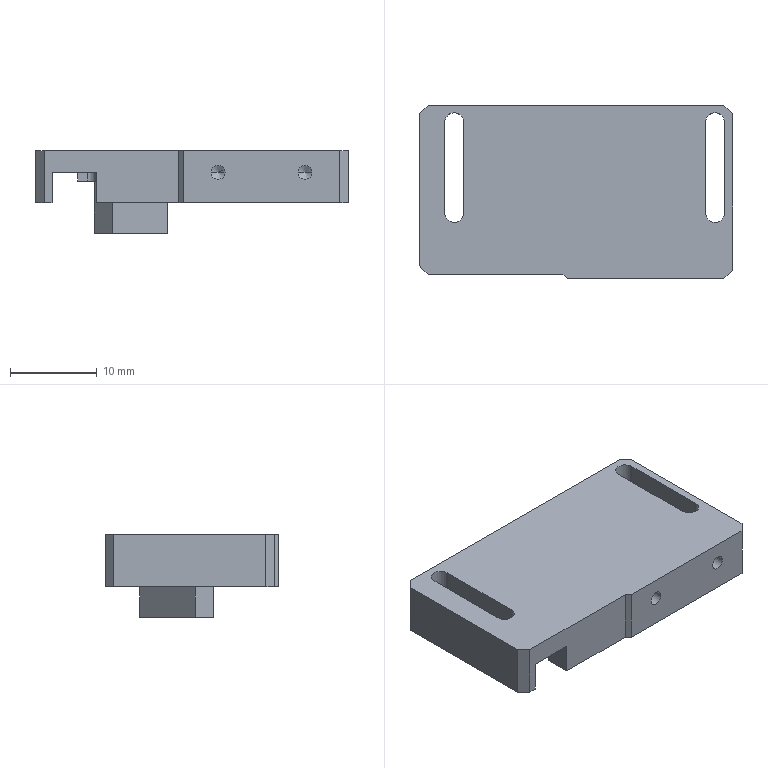NC program | NX | posted with a generic post | part box 36 x 20 x 9.5 mm
Lines 1630 to 2686 of 4561:
(CAVITY_MILL_COPY_COPY , TOOL : D2)
N3240 T02 M6
N3242 G54
N3244 G17 G0 G90 X9.747 Y2.177 S9974 M3
N3246 G43 Z30. H2
N3248 Z-2.092
N3250 G94 G1 Z-3.592 F1000.
N3252 X10.383 Y3.006
N3254 G3 X10.514 Y3.997 R1.
N3256 G1 X11.345 Y4.341
N3258 X11.406 Y4.178
N3260 X11.728 Y4.5
N3262 X11.273
N3264 X11.345 Y4.341
N3266 X10.514 Y3.997
N3268 G2 X10.408 Y2.593 R1.56
N3270 G3 X10.482 Y1.981 R0.5
N3272 G1 X13.122 Y4.621
N3274 G2 X14.745 Y4.548 R1.1
N3276 X15. Y3.828 R1.1
N3278 G1 Y3.39
N3280 G3 X15.485 Y3.771 R0.5
N3282 G2 X16.626 Y4.915 R1.56
N3284 G3 X17.006 Y5.4 R0.5
N3286 G1 X9.066
N3288 G3 X9.446 Y4.915 R0.5
N3290 G2 X10.514 Y3.997 R1.56
N3292 X10.383 Y3.006 R1.
N3294 G1 X9.747 Y2.177
N3296 Z-2.092
N3298 G0 Z-2.285
N3300 G1 Z-3.785
N3302 X10.383 Y3.006
N3304 G3 X10.514 Y3.997 R1.
N3306 G1 X11.345 Y4.341
N3308 X11.406 Y4.178
N3310 X11.728 Y4.5
N3312 X11.273
N3314 X11.345 Y4.341
N3316 X10.514 Y3.997
N3318 G2 X10.408 Y2.593 R1.56
N3320 G3 X10.482 Y1.981 R0.5
N3322 G1 X13.122 Y4.621
N3324 G2 X14.745 Y4.548 R1.1
N3326 X15. Y3.828 R1.1
N3328 G1 Y3.39
N3330 G3 X15.485 Y3.771 R0.5
N3332 G2 X16.626 Y4.915 R1.56
N3334 G3 X17.006 Y5.4 R0.5
N3336 G1 X9.066
N3338 G3 X9.446 Y4.915 R0.5
N3340 G2 X10.514 Y3.997 R1.56
N3342 X10.383 Y3.006 R1.
N3344 G1 X9.747 Y2.177
N3346 Z-2.285
N3348 G0 Z-2.477
N3350 G1 Z-3.977
N3352 X10.383 Y3.006
N3354 G3 X10.514 Y3.997 R1.
N3356 G1 X11.345 Y4.341
N3358 X11.406 Y4.178
N3360 X11.728 Y4.5
N3362 X11.273
N3364 X11.345 Y4.341
N3366 X10.514 Y3.997
N3368 G2 X10.408 Y2.593 R1.56
N3370 G3 X10.482 Y1.981 R0.5
N3372 G1 X13.122 Y4.621
N3374 G2 X14.745 Y4.548 R1.1
N3376 X15. Y3.828 R1.1
N3378 G1 Y3.39
N3380 G3 X15.485 Y3.771 R0.5
N3382 G2 X16.626 Y4.915 R1.56
N3384 G3 X17.006 Y5.4 R0.5
N3386 G1 X9.066
N3388 G3 X9.446 Y4.915 R0.5
N3390 G2 X10.514 Y3.997 R1.56
N3392 X10.383 Y3.006 R1.
N3394 G1 X9.747 Y2.177
N3396 Z-2.477
N3398 G0 Z-2.669
N3400 G1 Z-4.169
N3402 X10.383 Y3.006
N3404 G3 X10.514 Y3.997 R1.
N3406 G1 X11.345 Y4.341
N3408 X11.406 Y4.178
N3410 X11.728 Y4.5
N3412 X11.273
N3414 X11.345 Y4.341
N3416 X10.514 Y3.997
N3418 G2 X10.408 Y2.593 R1.56
N3420 G3 X10.482 Y1.981 R0.5
N3422 G1 X13.122 Y4.621
N3424 G2 X14.745 Y4.548 R1.1
N3426 X15. Y3.828 R1.1
N3428 G1 Y3.39
N3430 G3 X15.485 Y3.771 R0.5
N3432 G2 X16.626 Y4.915 R1.56
N3434 G3 X17.006 Y5.4 R0.5
N3436 G1 X9.066
N3438 G3 X9.446 Y4.915 R0.5
N3440 G2 X10.514 Y3.997 R1.56
N3442 X10.383 Y3.006 R1.
N3444 G1 X9.747 Y2.177
N3446 Z-2.669
N3448 G0 Z-2.862
N3450 G1 Z-4.362
N3452 X10.383 Y3.006
N3454 G3 X10.514 Y3.997 R1.
N3456 G1 X11.345 Y4.341
N3458 X11.406 Y4.178
N3460 X11.728 Y4.5
N3462 X11.273
N3464 X11.345 Y4.341
N3466 X10.514 Y3.997
N3468 G2 X10.408 Y2.593 R1.56
N3470 G3 X10.482 Y1.981 R0.5
N3472 G1 X13.122 Y4.621
N3474 G2 X14.745 Y4.548 R1.1
N3476 X15. Y3.828 R1.1
N3478 G1 Y3.39
N3480 G3 X15.485 Y3.771 R0.5
N3482 G2 X16.626 Y4.915 R1.56
N3484 G3 X17.006 Y5.4 R0.5
N3486 G1 X9.066
N3488 G3 X9.446 Y4.915 R0.5
N3490 G2 X10.514 Y3.997 R1.56
N3492 X10.383 Y3.006 R1.
N3494 G1 X9.747 Y2.177
N3496 Z-2.862
N3498 G0 Z-3.054
N3500 G1 Z-4.554
N3502 X10.383 Y3.006
N3504 G3 X10.514 Y3.997 R1.
N3506 G1 X11.345 Y4.341
N3508 X11.406 Y4.178
N3510 X11.728 Y4.5
N3512 X11.273
N3514 X11.345 Y4.341
N3516 X10.514 Y3.997
N3518 G2 X10.408 Y2.593 R1.56
N3520 G3 X10.482 Y1.981 R0.5
N3522 G1 X13.122 Y4.621
N3524 G2 X14.745 Y4.548 R1.1
N3526 X15. Y3.828 R1.1
N3528 G1 Y3.39
N3530 G3 X15.485 Y3.771 R0.5
N3532 G2 X16.626 Y4.915 R1.56
N3534 G3 X17.006 Y5.4 R0.5
N3536 G1 X9.066
N3538 G3 X9.446 Y4.915 R0.5
N3540 G2 X10.514 Y3.997 R1.56
N3542 X10.383 Y3.006 R1.
N3544 G1 X9.747 Y2.177
N3546 Z-3.054
N3548 G0 Z-3.246
N3550 G1 Z-4.746
N3552 X10.383 Y3.006
N3554 G3 X10.514 Y3.997 R1.
N3556 G1 X11.345 Y4.341
N3558 X11.406 Y4.178
N3560 X11.728 Y4.5
N3562 X11.273
N3564 X11.345 Y4.341
N3566 X10.514 Y3.997
N3568 G2 X10.408 Y2.593 R1.56
N3570 G3 X10.482 Y1.981 R0.5
N3572 G1 X13.122 Y4.621
N3574 G2 X14.745 Y4.548 R1.1
N3576 X15. Y3.828 R1.1
N3578 G1 Y3.39
N3580 G3 X15.485 Y3.771 R0.5
N3582 G2 X16.626 Y4.915 R1.56
N3584 G3 X17.006 Y5.4 R0.5
N3586 G1 X9.066
N3588 G3 X9.446 Y4.915 R0.5
N3590 G2 X10.514 Y3.997 R1.56
N3592 X10.383 Y3.006 R1.
N3594 G1 X9.747 Y2.177
N3596 Z-3.246
N3598 G0 Z-3.438
N3600 G1 Z-4.938
N3602 X10.383 Y3.006
N3604 G3 X10.514 Y3.997 R1.
N3606 G1 X11.345 Y4.341
N3608 X11.406 Y4.178
N3610 X11.728 Y4.5
N3612 X11.273
N3614 X11.345 Y4.341
N3616 X10.514 Y3.997
N3618 G2 X10.408 Y2.593 R1.56
N3620 G3 X10.482 Y1.981 R0.5
N3622 G1 X13.122 Y4.621
N3624 G2 X14.745 Y4.548 R1.1
N3626 X15. Y3.828 R1.1
N3628 G1 Y3.39
N3630 G3 X15.485 Y3.771 R0.5
N3632 G2 X16.626 Y4.915 R1.56
N3634 G3 X17.006 Y5.4 R0.5
N3636 G1 X9.066
N3638 G3 X9.446 Y4.915 R0.5
N3640 G2 X10.514 Y3.997 R1.56
N3642 X10.383 Y3.006 R1.
N3644 G1 X9.747 Y2.177
N3646 Z-3.438
N3648 G0 Z-3.631
N3650 G1 Z-5.131
N3652 X10.383 Y3.006
N3654 G3 X10.514 Y3.997 R1.
N3656 G1 X11.345 Y4.341
N3658 X11.406 Y4.178
N3660 X11.728 Y4.5
N3662 X11.273
N3664 X11.345 Y4.341
N3666 X10.514 Y3.997
N3668 G2 X10.408 Y2.593 R1.56
N3670 G3 X10.482 Y1.981 R0.5
N3672 G1 X13.122 Y4.621
N3674 G2 X14.745 Y4.548 R1.1
N3676 X15. Y3.828 R1.1
N3678 G1 Y3.39
N3680 G3 X15.485 Y3.771 R0.5
N3682 G2 X16.626 Y4.915 R1.56
N3684 G3 X17.006 Y5.4 R0.5
N3686 G1 X9.066
N3688 G3 X9.446 Y4.915 R0.5
N3690 G2 X10.514 Y3.997 R1.56
N3692 X10.383 Y3.006 R1.
N3694 G1 X9.747 Y2.177
N3696 Z-3.631
N3698 G0 Z-3.823
N3700 G1 Z-5.323
N3702 X10.383 Y3.006
N3704 G3 X10.514 Y3.997 R1.
N3706 G1 X11.345 Y4.341
N3708 X11.406 Y4.178
N3710 X11.728 Y4.5
N3712 X11.273
N3714 X11.345 Y4.341
N3716 X10.514 Y3.997
N3718 G2 X10.408 Y2.593 R1.56
N3720 G3 X10.482 Y1.981 R0.5
N3722 G1 X13.122 Y4.621
N3724 G2 X14.745 Y4.548 R1.1
N3726 X15. Y3.828 R1.1
N3728 G1 Y3.39
N3730 G3 X15.485 Y3.771 R0.5
N3732 G2 X16.626 Y4.915 R1.56
N3734 G3 X17.006 Y5.4 R0.5
N3736 G1 X9.066
N3738 G3 X9.446 Y4.915 R0.5
N3740 G2 X10.514 Y3.997 R1.56
N3742 X10.383 Y3.006 R1.
N3744 G1 X9.747 Y2.177
N3746 Z-3.823
N3748 G0 Z-4.015
N3750 G1 Z-5.515
N3752 X10.383 Y3.006
N3754 G3 X10.514 Y3.997 R1.
N3756 G1 X11.345 Y4.341
N3758 X11.406 Y4.178
N3760 X11.728 Y4.5
N3762 X11.273
N3764 X11.345 Y4.341
N3766 X10.514 Y3.997
N3768 G2 X10.408 Y2.593 R1.56
N3770 G3 X10.482 Y1.981 R0.5
N3772 G1 X13.122 Y4.621
N3774 G2 X14.745 Y4.548 R1.1
N3776 X15. Y3.828 R1.1
N3778 G1 Y3.39
N3780 G3 X15.485 Y3.771 R0.5
N3782 G2 X16.626 Y4.915 R1.56
N3784 G3 X17.006 Y5.4 R0.5
N3786 G1 X9.066
N3788 G3 X9.446 Y4.915 R0.5
N3790 G2 X10.514 Y3.997 R1.56
N3792 X10.383 Y3.006 R1.
N3794 G1 X9.747 Y2.177
N3796 Z-4.015
N3798 G0 Z-4.208
N3800 G1 Z-5.708
N3802 X10.383 Y3.006
N3804 G3 X10.514 Y3.997 R1.
N3806 G1 X11.345 Y4.341
N3808 X11.406 Y4.178
N3810 X11.728 Y4.5
N3812 X11.273
N3814 X11.345 Y4.341
N3816 X10.514 Y3.997
N3818 G2 X10.408 Y2.593 R1.56
N3820 G3 X10.482 Y1.981 R0.5
N3822 G1 X13.122 Y4.621
N3824 G2 X14.745 Y4.548 R1.1
N3826 X15. Y3.828 R1.1
N3828 G1 Y3.39
N3830 G3 X15.485 Y3.771 R0.5
N3832 G2 X16.626 Y4.915 R1.56
N3834 G3 X17.006 Y5.4 R0.5
N3836 G1 X9.066
N3838 G3 X9.446 Y4.915 R0.5
N3840 G2 X10.514 Y3.997 R1.56
N3842 X10.383 Y3.006 R1.
N3844 G1 X9.747 Y2.177
N3846 Z-4.208
N3848 G0 Z-4.4
N3850 G1 Z-5.9
N3852 X10.383 Y3.006
N3854 G3 X10.514 Y3.997 R1.
N3856 G1 X11.345 Y4.341
N3858 X11.406 Y4.178
N3860 X11.728 Y4.5
N3862 X11.273
N3864 X11.345 Y4.341
N3866 X10.514 Y3.997
N3868 G2 X10.408 Y2.593 R1.56
N3870 G3 X10.482 Y1.981 R0.5
N3872 G1 X13.122 Y4.621
N3874 G2 X14.745 Y4.548 R1.1
N3876 X15. Y3.828 R1.1
N3878 G1 Y3.39
N3880 G3 X15.485 Y3.771 R0.5
N3882 G2 X16.626 Y4.915 R1.56
N3884 G3 X17.006 Y5.4 R0.5
N3886 G1 X9.066
N3888 G3 X9.446 Y4.915 R0.5
N3890 G2 X10.514 Y3.997 R1.56
N3892 X10.383 Y3.006 R1.
N3894 G1 X9.747 Y2.177
N3896 Z-4.4
N3898 G0 Z30.
N3900 X17.93 Y4.8
N3902 Z-4.6
N3904 G1 Z-6.1
N3906 X17.872 Y4.9
N3908 G3 X17.006 Y5.4 R1.
N3910 G1 X15.598
N3912 X14.745 Y4.548
N3914 G2 X15. Y3.828 R1.1
N3916 G1 Y3.39
N3918 G3 X15.5 Y2.524 R1.
N3920 G1 X15.6 Y2.466
N3922 Z-4.6
N3924 G0 X17.93 Y4.8 Z-4.8
N3926 G1 Z-6.3
N3928 X17.872 Y4.9
N3930 G3 X17.006 Y5.4 R1.
N3932 G1 X15.598
N3934 X14.745 Y4.548
N3936 G2 X15. Y3.828 R1.1
N3938 G1 Y3.39
N3940 G3 X15.5 Y2.524 R1.
N3942 G1 X15.6 Y2.466
N3944 Z-4.8
N3946 G0 X17.93 Y4.8 Z-5.
N3948 G1 Z-6.5
N3950 X17.872 Y4.9
N3952 G3 X17.006 Y5.4 R1.
N3954 G1 X15.598
N3956 X14.745 Y4.548
N3958 G2 X15. Y3.828 R1.1
N3960 G1 Y3.39
N3962 G3 X15.5 Y2.524 R1.
N3964 G1 X15.6 Y2.466
N3966 Z-5.
N3968 G0 X17.93 Y4.8 Z-5.2
N3970 G1 Z-6.7
N3972 X17.872 Y4.9
N3974 G3 X17.006 Y5.4 R1.
N3976 G1 X15.598
N3978 X14.745 Y4.548
N3980 G2 X15. Y3.828 R1.1
N3982 G1 Y3.39
N3984 G3 X15.5 Y2.524 R1.
N3986 G1 X15.6 Y2.466
N3988 Z-5.2
N3990 G0 X17.93 Y4.8 Z-5.4
N3992 G1 Z-6.9
N3994 X17.872 Y4.9
N3996 G3 X17.006 Y5.4 R1.
N3998 G1 X15.598
N4000 X14.745 Y4.548
N4002 G2 X15. Y3.828 R1.1
N4004 G1 Y3.39
N4006 G3 X15.5 Y2.524 R1.
N4008 G1 X15.6 Y2.466
N4010 Z-5.4
N4012 G0 Z30.
N4014 X9.142 Y-5.614
N4016 Z-4.6
N4018 G1 Z-6.1
N4020 X9.006 Y-4.578
N4022 G3 X8.397 Y-3.785 R1.
N4024 G1 X8.741 Y-2.953
N4026 X8.9 Y-3.026
N4028 Y-2.571
N4030 X8.578 Y-2.892
N4032 X8.741 Y-2.953
N4034 X8.397 Y-3.785
N4036 G2 X9.315 Y-4.852 R1.56
N4038 G3 X9.8 Y-5.233 R0.5
N4040 G1 Y-0.398
N4042 X6.381 Y-3.817
N4044 G3 X6.993 Y-3.891 R0.5
N4046 G2 X8.397 Y-3.785 R1.56
N4048 X9.006 Y-4.578 R1.
N4050 G1 X9.142 Y-5.614
N4052 Z-4.6
N4054 G0 Z-4.8
N4056 G1 Z-6.3
N4058 X9.006 Y-4.578
N4060 G3 X8.397 Y-3.785 R1.
N4062 G1 X8.741 Y-2.953
N4064 X8.9 Y-3.026
N4066 Y-2.571
N4068 X8.578 Y-2.892
N4070 X8.741 Y-2.953
N4072 X8.397 Y-3.785
N4074 G2 X9.315 Y-4.852 R1.56
N4076 G3 X9.8 Y-5.233 R0.5
N4078 G1 Y-0.398
N4080 X6.381 Y-3.817
N4082 G3 X6.993 Y-3.891 R0.5
N4084 G2 X8.397 Y-3.785 R1.56
N4086 X9.006 Y-4.578 R1.
N4088 G1 X9.142 Y-5.614
N4090 Z-4.8
N4092 G0 Z-5.
N4094 G1 Z-6.5
N4096 X9.006 Y-4.578
N4098 G3 X8.397 Y-3.785 R1.
N4100 G1 X8.741 Y-2.953
N4102 X8.9 Y-3.026
N4104 Y-2.571
N4106 X8.578 Y-2.892
N4108 X8.741 Y-2.953
N4110 X8.397 Y-3.785
N4112 G2 X9.315 Y-4.852 R1.56
N4114 G3 X9.8 Y-5.233 R0.5
N4116 G1 Y-0.398
N4118 X6.381 Y-3.817
N4120 G3 X6.993 Y-3.891 R0.5
N4122 G2 X8.397 Y-3.785 R1.56
N4124 X9.006 Y-4.578 R1.
N4126 G1 X9.142 Y-5.614
N4128 Z-5.
N4130 G0 Z-5.2
N4132 G1 Z-6.7
N4134 X9.006 Y-4.578
N4136 G3 X8.397 Y-3.785 R1.
N4138 G1 X8.741 Y-2.953
N4140 X8.9 Y-3.026
N4142 Y-2.571
N4144 X8.578 Y-2.892
N4146 X8.741 Y-2.953
N4148 X8.397 Y-3.785
N4150 G2 X9.315 Y-4.852 R1.56
N4152 G3 X9.8 Y-5.233 R0.5
N4154 G1 Y-0.398
N4156 X6.381 Y-3.817
N4158 G3 X6.993 Y-3.891 R0.5
N4160 G2 X8.397 Y-3.785 R1.56
N4162 X9.006 Y-4.578 R1.
N4164 G1 X9.142 Y-5.614
N4166 Z-5.2
N4168 G0 Z-5.4
N4170 G1 Z-6.9
N4172 X9.006 Y-4.578
N4174 G3 X8.397 Y-3.785 R1.
N4176 G1 X8.741 Y-2.953
N4178 X8.9 Y-3.026
N4180 Y-2.571
N4182 X8.578 Y-2.892
N4184 X8.741 Y-2.953
N4186 X8.397 Y-3.785
N4188 G2 X9.315 Y-4.852 R1.56
N4190 G3 X9.8 Y-5.233 R0.5
N4192 G1 Y-0.398
N4194 X6.381 Y-3.817
N4196 G3 X6.993 Y-3.891 R0.5
N4198 G2 X8.397 Y-3.785 R1.56
N4200 X9.006 Y-4.578 R1.
N4202 G1 X9.142 Y-5.614
N4204 Z-5.4
N4206 G0 Z30.
N4208 X-1.132 Y-7.915
N4210 Z-4.6
N4212 G1 Z-6.1
N4214 X-1.102 Y-7.803
N4216 G3 X-1.361 Y-6.837 R1.
N4218 G1 X-2.778 Y-5.42
N4220 X-4.122 Y-6.763
N4222 X-4.196 Y-6.831
N4224 G3 X-4.554 Y-7.65 R1.
N4226 G1 Z-4.6
N4228 G0 X-1.132 Y-7.915 Z-4.8
N4230 G1 Z-6.3
N4232 X-1.102 Y-7.803
N4234 G3 X-1.361 Y-6.837 R1.
N4236 G1 X-2.778 Y-5.42
N4238 X-4.122 Y-6.763
N4240 X-4.196 Y-6.831
N4242 G3 X-4.554 Y-7.65 R1.
N4244 G1 Z-4.8
N4246 G0 X-1.132 Y-7.915 Z-5.
N4248 G1 Z-6.5
N4250 X-1.102 Y-7.803
N4252 G3 X-1.361 Y-6.837 R1.
N4254 G1 X-2.778 Y-5.42
N4256 X-4.122 Y-6.763
N4258 X-4.196 Y-6.831
N4260 G3 X-4.554 Y-7.65 R1.
N4262 G1 Z-5.
N4264 G0 X-1.132 Y-7.915 Z-5.2
N4266 G1 Z-6.7
N4268 X-1.102 Y-7.803
N4270 G3 X-1.361 Y-6.837 R1.
N4272 G1 X-2.778 Y-5.42
N4274 X-4.122 Y-6.763
N4276 X-4.196 Y-6.831
N4278 G3 X-4.554 Y-7.65 R1.
N4280 G1 Z-5.2
N4282 G0 X-1.132 Y-7.915 Z-5.4
N4284 G1 Z-6.9
N4286 X-1.102 Y-7.803
N4288 G3 X-1.361 Y-6.837 R1.
N4290 G1 X-2.778 Y-5.42
N4292 X-4.122 Y-6.763
N4294 X-4.196 Y-6.831
N4296 G3 X-4.554 Y-7.65 R1.
N4298 G1 Z-5.4
N4300 G0 Z30.
N4302 X-3.618 Y11.2
N4304 Z-2.092
N4306 G1 Z-3.592
N4308 X-3.56 Y11.1
N4310 G3 X-2.694 Y10.6 R1.
N4312 G1 X-1.956
N4314 X-1.778 Y10.778
N4316 G2 X-1.419 Y11.017 R1.1
N4318 G3 X-0.829 Y11.7 R1.
N4320 G1 Z-2.092
N4322 G0 X-3.618 Y11.2 Z-2.285
N4324 G1 Z-3.785
N4326 X-3.56 Y11.1
N4328 G3 X-2.694 Y10.6 R1.
N4330 G1 X-1.956
N4332 X-1.778 Y10.778
N4334 G2 X-1.419 Y11.017 R1.1
N4336 G3 X-0.829 Y11.7 R1.
N4338 G1 Z-2.285
N4340 G0 X-3.618 Y11.2 Z-2.477
N4342 G1 Z-3.977
N4344 X-3.56 Y11.1
N4346 G3 X-2.694 Y10.6 R1.
N4348 G1 X-1.956
N4350 X-1.778 Y10.778
N4352 G2 X-1.419 Y11.017 R1.1
N4354 G3 X-0.829 Y11.7 R1.
N4356 G1 Z-2.477
N4358 G0 X-3.618 Y11.2 Z-2.669
N4360 G1 Z-4.169
N4362 X-3.56 Y11.1
N4364 G3 X-2.694 Y10.6 R1.
N4366 G1 X-1.956
N4368 X-1.778 Y10.778
N4370 G2 X-1.419 Y11.017 R1.1
N4372 G3 X-0.829 Y11.7 R1.
N4374 G1 Z-2.669
N4376 G0 X-3.618 Y11.2 Z-2.862
N4378 G1 Z-4.362
N4380 X-3.56 Y11.1
N4382 G3 X-2.694 Y10.6 R1.
N4384 G1 X-1.956
N4386 X-1.778 Y10.778
N4388 G2 X-1.419 Y11.017 R1.1
N4390 G3 X-0.829 Y11.7 R1.
N4392 G1 Z-2.862
N4394 G0 X-3.618 Y11.2 Z-3.054
N4396 G1 Z-4.554
N4398 X-3.56 Y11.1
N4400 G3 X-2.694 Y10.6 R1.
N4402 G1 X-1.956
N4404 X-1.778 Y10.778
N4406 G2 X-1.419 Y11.017 R1.1
N4408 G3 X-0.829 Y11.7 R1.
N4410 G1 Z-3.054
N4412 G0 X-3.618 Y11.2 Z-3.246
N4414 G1 Z-4.746
N4416 X-3.56 Y11.1
N4418 G3 X-2.694 Y10.6 R1.
N4420 G1 X-1.956
N4422 X-1.778 Y10.778
N4424 G2 X-1.419 Y11.017 R1.1
N4426 G3 X-0.829 Y11.7 R1.
N4428 G1 Z-3.246
N4430 G0 X-3.618 Y11.2 Z-3.438
N4432 G1 Z-4.938
N4434 X-3.56 Y11.1
N4436 G3 X-2.694 Y10.6 R1.
N4438 G1 X-1.956
N4440 X-1.778 Y10.778
N4442 G2 X-1.419 Y11.017 R1.1
N4444 G3 X-0.829 Y11.7 R1.
N4446 G1 Z-3.438
N4448 G0 X-3.618 Y11.2 Z-3.631
N4450 G1 Z-5.131
N4452 X-3.56 Y11.1
N4454 G3 X-2.694 Y10.6 R1.
N4456 G1 X-1.956
N4458 X-1.778 Y10.778
N4460 G2 X-1.419 Y11.017 R1.1
N4462 G3 X-0.829 Y11.7 R1.
N4464 G1 Z-3.631
N4466 G0 X-3.618 Y11.2 Z-3.823
N4468 G1 Z-5.323
N4470 X-3.56 Y11.1
N4472 G3 X-2.694 Y10.6 R1.
N4474 G1 X-1.956
N4476 X-1.778 Y10.778
N4478 G2 X-1.419 Y11.017 R1.1
N4480 G3 X-0.829 Y11.7 R1.
N4482 G1 Z-3.823
N4484 G0 X-3.618 Y11.2 Z-4.015
N4486 G1 Z-5.515
N4488 X-3.56 Y11.1
N4490 G3 X-2.694 Y10.6 R1.
N4492 G1 X-1.956
N4494 X-1.778 Y10.778
N4496 G2 X-1.419 Y11.017 R1.1
N4498 G3 X-0.829 Y11.7 R1.
N4500 G1 Z-4.015
N4502 G0 X-3.618 Y11.2 Z-4.208
N4504 G1 Z-5.708
N4506 X-3.56 Y11.1
N4508 G3 X-2.694 Y10.6 R1.
N4510 G1 X-1.956
N4512 X-1.778 Y10.778
N4514 G2 X-1.419 Y11.017 R1.1
N4516 G3 X-0.829 Y11.7 R1.
N4518 G1 Z-4.208
N4520 G0 X-3.618 Y11.2 Z-4.4
N4522 G1 Z-5.9
N4524 X-3.56 Y11.1
N4526 G3 X-2.694 Y10.6 R1.
N4528 G1 X-1.956
N4530 X-1.778 Y10.778
N4532 G2 X-1.419 Y11.017 R1.1
N4534 G3 X-0.829 Y11.7 R1.
N4536 G1 Z-4.4
N4538 G0 X-3.618 Y11.2 Z-4.6
N4540 G1 Z-6.1
N4542 X-3.56 Y11.1
N4544 G3 X-2.694 Y10.6 R1.
N4546 G1 X-1.956
N4548 X-1.778 Y10.778
N4550 G2 X-1.419 Y11.017 R1.1
N4552 G3 X-0.829 Y11.7 R1.
N4554 G1 Z-4.6
N4556 G0 X-3.618 Y11.2 Z-4.8
N4558 G1 Z-6.3
N4560 X-3.561 Y11.1
N4562 G3 X-2.694 Y10.6 R1.
N4564 G1 X-1.956
N4566 X-1.778 Y10.778
N4568 G2 X-1.419 Y11.017 R1.1
N4570 G3 X-0.829 Y11.7 R1.
N4572 G1 Z-4.8
N4574 G0 X-3.618 Y11.2 Z-5.
N4576 G1 Z-6.5
N4578 X-3.561 Y11.1
N4580 G3 X-2.694 Y10.6 R1.
N4582 G1 X-1.956
N4584 X-1.778 Y10.778
N4586 G2 X-1.419 Y11.017 R1.1
N4588 G3 X-0.829 Y11.7 R1.
N4590 G1 Z-5.
N4592 G0 X-3.618 Y11.2 Z-5.2
N4594 G1 Z-6.7
N4596 X-3.561 Y11.1
N4598 G3 X-2.695 Y10.6 R1.
N4600 G1 X-1.956
N4602 X-1.778 Y10.778
N4604 G2 X-1.419 Y11.017 R1.1
N4606 G3 X-0.829 Y11.7 R1.
N4608 G1 Z-5.2
N4610 G0 X-3.618 Y11.2 Z-5.4
N4612 G1 Z-6.9
N4614 X-3.561 Y11.1
N4616 G3 X-2.695 Y10.6 R1.
N4618 G1 X-1.956
N4620 X-1.778 Y10.778
N4622 G2 X-1.419 Y11.017 R1.1
N4624 G3 X-0.829 Y11.7 R1.
N4626 G1 Z-5.4
N4628 G0 X-3.618 Y11.2 Z-5.6
N4630 G1 Z-7.1
N4632 X-3.561 Y11.1
N4634 G3 X-2.695 Y10.6 R1.
N4636 G1 X-1.956
N4638 X-1.778 Y10.778
N4640 G2 X-1.419 Y11.017 R1.1
N4642 G3 X-0.829 Y11.7 R1.
N4644 G1 Z-5.6
N4646 G0 X-3.618 Y11.2 Z-5.8
N4648 G1 Z-7.3
N4650 X-3.561 Y11.1
N4652 G3 X-2.695 Y10.6 R1.
N4654 G1 X-1.956
N4656 X-1.778 Y10.778
N4658 G2 X-1.419 Y11.017 R1.1
N4660 G3 X-0.829 Y11.7 R1.
N4662 G1 Z-5.8
N4664 G0 X-3.618 Y11.2 Z-6.
N4666 G1 Z-7.5
N4668 X-3.561 Y11.1
N4670 G3 X-2.695 Y10.6 R1.
N4672 G1 X-1.956
N4674 X-1.778 Y10.778
N4676 G2 X-1.419 Y11.017 R1.1
N4678 G3 X-0.829 Y11.7 R1.
N4680 G1 Z-6.
N4682 G0 X-3.618 Y11.2 Z-6.2
N4684 G1 Z-7.7
N4686 X-3.561 Y11.1
N4688 G3 X-2.695 Y10.6 R1.
N4690 G1 X-1.956
N4692 X-1.778 Y10.778
N4694 G2 X-1.419 Y11.017 R1.1
N4696 G3 X-0.829 Y11.7 R1.
N4698 G1 Z-6.2
N4700 G0 X-3.618 Y11.2 Z-6.4
N4702 G1 Z-7.9
N4704 X-3.561 Y11.1
N4706 G3 X-2.695 Y10.6 R1.
N4708 G1 X-1.956
N4710 X-1.778 Y10.778
N4712 G2 X-1.419 Y11.017 R1.1
N4714 G3 X-0.829 Y11.7 R1.
N4716 G1 Z-6.4
N4718 G0 X-3.618 Y11.2 Z-6.6
N4720 G1 Z-8.1
N4722 X-3.561 Y11.1
N4724 G3 X-2.695 Y10.6 R1.
N4726 G1 X-1.956
N4728 X-1.778 Y10.778
N4730 G2 X-1.419 Y11.017 R1.1
N4732 G3 X-0.829 Y11.7 R1.
N4734 G1 Z-6.6
N4736 G0 X-3.618 Y11.2 Z-6.8
N4738 G1 Z-8.3
N4740 X-3.561 Y11.1
N4742 G3 X-2.695 Y10.6 R1.
N4744 G1 X-1.956
N4746 X-1.778 Y10.778
N4748 G2 X-1.419 Y11.017 R1.1
N4750 G3 X-0.829 Y11.7 R1.
N4752 G1 Z-6.8
N4754 G0 X-3.618 Y11.2 Z-7.
N4756 G1 Z-8.5
N4758 X-3.561 Y11.1
N4760 G3 X-2.695 Y10.6 R1.
N4762 G1 X-1.956
N4764 X-1.778 Y10.778
N4766 G2 X-1.419 Y11.017 R1.1
N4768 G3 X-0.829 Y11.7 R1.
N4770 G1 Z-7.
N4772 G0 X-3.618 Y11.2 Z-7.2
N4774 G1 Z-8.7
N4776 X-3.561 Y11.1
N4778 G3 X-2.695 Y10.6 R1.
N4780 G1 X-1.956
N4782 X-1.778 Y10.778
N4784 G2 X-1.419 Y11.017 R1.1
N4786 G3 X-0.829 Y11.7 R1.
N4788 G1 Z-7.2
N4790 G0 X-3.618 Y11.2 Z-7.4
N4792 G1 Z-8.9
N4794 X-3.561 Y11.1
N4796 G3 X-2.695 Y10.6 R1.
N4798 G1 X-1.956
N4800 X-1.778 Y10.778
N4802 G2 X-1.419 Y11.017 R1.1
N4804 G3 X-0.829 Y11.7 R1.
N4806 G1 Z-7.4
N4808 G0 X-3.618 Y11.2 Z-7.6
N4810 G1 Z-9.1
N4812 X-3.561 Y11.1
N4814 G3 X-2.695 Y10.6 R1.
N4816 G1 X-1.956
N4818 X-1.778 Y10.778
N4820 G2 X-1.419 Y11.017 R1.1
N4822 G3 X-0.829 Y11.7 R1.
N4824 G1 Z-7.6
N4826 G0 X-3.618 Y11.2 Z-7.8
N4828 G1 Z-9.3
N4830 X-3.561 Y11.1
N4832 G3 X-2.695 Y10.6 R1.
N4834 G1 X-1.956
N4836 X-1.778 Y10.778
N4838 G2 X-1.419 Y11.017 R1.1
N4840 G3 X-0.829 Y11.7 R1.
N4842 G1 Z-7.8
N4844 G0 X-3.618 Y11.2 Z-8.
N4846 G1 Z-9.5
N4848 X-3.561 Y11.1
N4850 G3 X-2.695 Y10.6 R1.
N4852 G1 X-1.956
N4854 X-1.778 Y10.778
N4856 G2 X-1.419 Y11.017 R1.1
N4858 G3 X-0.829 Y11.7 R1.
N4860 G1 Z-8.
N4862 G0 Z30.
N4864 X-14.795 Y10.961
N4866 Z-2.092
N4868 G1 Z-3.592
N4870 X-14.397 Y10.254
N4872 G3 X-13.536 Y9.746 R1.
N4874 G1 X-13.55 Y8.346
N4876 X-13.6 Y8.347
N4878 Y6.995
N4880 X-13.5 Y7.014
N4882 Y8.346
N4884 X-13.55
N4886 X-13.536 Y9.746
N4888 X-13.562
N4890 G2 X-14.139 Y9.874 R1.56
N4892 G1 X-14.227 Y9.912
N4894 G2 X-14.718 Y10.248 R1.56
N4896 G3 X-15.355 Y10.31 R0.5
N4898 G2 X-15. Y9.5 R1.1
N4900 G1 Y4.09
N4902 G3 X-14.515 Y4.471 R0.5
N4904 G2 X-12.205 Y5.439 R1.56
N4906 G1 X-12.117 Y5.387
N4908 G3 X-11.686 Y5.349 R0.5
N4910 X-11.467 Y5. R0.5
N4912 G2 X-10.992 Y2.892 R1.56
N4914 G3 X-10.918 Y2.28 R0.5
N4916 G1 X-9.92 Y3.278
N4918 G2 X-8.364 Y3.278 R1.1
N4920 G1 X-7.068 Y1.981
N4922 G3 X-6.993 Y2.593 R0.5
N4924 G2 X-6.032 Y4.915 R1.56
N4926 G3 X-5.652 Y5.4 R0.5
N4928 G1 X-8.248
N4930 X-8.105 Y4.366
N4932 X-8.248 Y5.4
N4934 X-11.
N4936 G2 X-12.1 Y6.5 R1.1
N4938 G1 Y9.5
N4940 G2 X-11.757 Y10.298 R1.1
N4942 G3 X-12.393 Y10.227 R0.5
N4944 G2 X-13.536 Y9.746 R1.56
N4946 X-14.397 Y10.254 R1.
N4948 G1 X-14.795 Y10.961
N4950 Z-2.092
N4952 G0 Z-2.285
N4954 G1 Z-3.785
N4956 X-14.397 Y10.254
N4958 G3 X-13.536 Y9.746 R1.
N4960 G1 X-13.55 Y8.346
N4962 X-13.6 Y8.347
N4964 Y6.995
N4966 X-13.5 Y7.014
N4968 Y8.346
N4970 X-13.55
N4972 X-13.536 Y9.746
N4974 X-13.562
N4976 G2 X-14.139 Y9.874 R1.56
N4978 G1 X-14.227 Y9.912
N4980 G2 X-14.718 Y10.248 R1.56
N4982 G3 X-15.355 Y10.31 R0.5
N4984 G2 X-15. Y9.5 R1.1
N4986 G1 Y4.09
N4988 G3 X-14.515 Y4.471 R0.5
N4990 G2 X-12.205 Y5.439 R1.56
N4992 G1 X-12.117 Y5.387
N4994 G3 X-11.686 Y5.349 R0.5
N4996 X-11.467 Y5. R0.5
N4998 G2 X-10.992 Y2.892 R1.56
N5000 G3 X-10.918 Y2.28 R0.5
N5002 G1 X-9.92 Y3.278
N5004 G2 X-8.674 Y3.495 R1.1
N5006 G1 X-8.105 Y4.366
N5008 X-8.674 Y3.495
N5010 G2 X-8.364 Y3.278 R1.1
N5012 G1 X-7.068 Y1.981
N5014 G3 X-6.993 Y2.593 R0.5
N5016 G2 X-6.032 Y4.915 R1.56
N5018 G3 X-5.652 Y5.4 R0.5
N5020 G1 X-11.
N5022 G2 X-12.1 Y6.5 R1.1
N5024 G1 Y9.5
N5026 G2 X-11.757 Y10.298 R1.1
N5028 G3 X-12.393 Y10.227 R0.5
N5030 G2 X-13.536 Y9.746 R1.56
N5032 X-14.397 Y10.254 R1.
N5034 G1 X-14.795 Y10.961
N5036 Z-2.285
N5038 G0 Z-2.477
N5040 G1 Z-3.977
N5042 X-14.397 Y10.254
N5044 G3 X-13.536 Y9.746 R1.
N5046 G1 X-13.55 Y8.346
N5048 X-13.6 Y8.347
N5050 Y6.995
N5052 X-13.5 Y7.014
N5054 Y8.346
N5056 X-13.55
N5058 X-13.536 Y9.746
N5060 X-13.562
N5062 G2 X-14.139 Y9.874 R1.56
N5064 G1 X-14.227 Y9.912
N5066 G2 X-14.718 Y10.248 R1.56
N5068 G3 X-15.355 Y10.31 R0.5
N5070 G2 X-15. Y9.5 R1.1
N5072 G1 Y4.09
N5074 G3 X-14.515 Y4.471 R0.5
N5076 G2 X-12.205 Y5.439 R1.56
N5078 G1 X-12.117 Y5.387
N5080 G3 X-11.686 Y5.349 R0.5
N5082 X-11.467 Y5. R0.5
N5084 G2 X-10.992 Y2.892 R1.56
N5086 G3 X-10.918 Y2.28 R0.5
N5088 G1 X-9.92 Y3.278
N5090 G2 X-8.674 Y3.495 R1.1
N5092 G1 X-8.105 Y4.366
N5094 X-8.674 Y3.495
N5096 G2 X-8.364 Y3.278 R1.1
N5098 G1 X-7.068 Y1.981
N5100 G3 X-6.993 Y2.593 R0.5
N5102 G2 X-6.032 Y4.915 R1.56
N5104 G3 X-5.652 Y5.4 R0.5
N5106 G1 X-11.
N5108 G2 X-12.1 Y6.5 R1.1
N5110 G1 Y9.5
N5112 G2 X-11.757 Y10.298 R1.1
N5114 G3 X-12.393 Y10.227 R0.5
N5116 G2 X-13.536 Y9.746 R1.56
N5118 X-14.397 Y10.254 R1.
N5120 G1 X-14.795 Y10.961
N5122 Z-2.477
N5124 G0 Z-2.669
N5126 G1 Z-4.169
N5128 X-14.397 Y10.254
N5130 G3 X-13.536 Y9.746 R1.
N5132 G1 X-13.55 Y8.346
N5134 X-13.6 Y8.347
N5136 Y6.995
N5138 X-13.5 Y7.014
N5140 Y8.346
N5142 X-13.55
N5144 X-13.536 Y9.746
N5146 X-13.562
N5148 G2 X-14.139 Y9.874 R1.56
N5150 G1 X-14.227 Y9.912
N5152 G2 X-14.718 Y10.248 R1.56
N5154 G3 X-15.355 Y10.31 R0.5
N5156 G2 X-15. Y9.5 R1.1
N5158 G1 Y4.09
N5160 G3 X-14.515 Y4.471 R0.5
N5162 G2 X-12.205 Y5.439 R1.56
N5164 G1 X-12.117 Y5.387
N5166 G3 X-11.686 Y5.349 R0.5
N5168 X-11.467 Y5. R0.5
N5170 G2 X-10.992 Y2.892 R1.56
N5172 G3 X-10.918 Y2.28 R0.5
N5174 G1 X-9.92 Y3.278
N5176 G2 X-8.364 Y3.278 R1.1
N5178 G1 X-7.068 Y1.981
N5180 G3 X-6.993 Y2.593 R0.5
N5182 G2 X-6.032 Y4.915 R1.56
N5184 G3 X-5.652 Y5.4 R0.5
N5186 G1 X-8.248
N5188 X-8.105 Y4.366
N5190 X-8.248 Y5.4
N5192 X-11.
N5194 G2 X-12.1 Y6.5 R1.1
N5196 G1 Y9.5
N5198 G2 X-11.757 Y10.298 R1.1
N5200 G3 X-12.393 Y10.227 R0.5
N5202 G2 X-13.536 Y9.746 R1.56
N5204 X-14.397 Y10.254 R1.
N5206 G1 X-14.795 Y10.961
N5208 Z-2.669
N5210 G0 Z-2.862
N5212 G1 Z-4.362
N5214 X-14.397 Y10.254
N5216 G3 X-13.536 Y9.746 R1.
N5218 G1 X-13.55 Y8.346
N5220 X-13.6 Y8.347
N5222 Y6.995
N5224 X-13.5 Y7.014
N5226 Y8.346
N5228 X-13.55
N5230 X-13.536 Y9.746
N5232 X-13.562
N5234 G2 X-14.139 Y9.874 R1.56
N5236 G1 X-14.227 Y9.912
N5238 G2 X-14.718 Y10.248 R1.56
N5240 G3 X-15.355 Y10.31 R0.5
N5242 G2 X-15. Y9.5 R1.1
N5244 G1 Y4.09
N5246 G3 X-14.515 Y4.47 R0.5
N5248 G2 X-12.205 Y5.439 R1.56
N5250 G1 X-12.117 Y5.387
N5252 G3 X-11.686 Y5.349 R0.5
N5254 X-11.467 Y5. R0.5
N5256 G2 X-10.992 Y2.892 R1.56
N5258 G3 X-10.918 Y2.28 R0.5
N5260 G1 X-9.92 Y3.278
N5262 G2 X-8.364 Y3.278 R1.1
N5264 G1 X-7.068 Y1.981
N5266 G3 X-6.993 Y2.593 R0.5
N5268 G2 X-6.032 Y4.915 R1.56
N5270 G3 X-5.652 Y5.4 R0.5
N5272 G1 X-8.248
N5274 X-8.105 Y4.366
N5276 X-8.248 Y5.4
N5278 X-11.
N5280 G2 X-12.1 Y6.5 R1.1
N5282 G1 Y9.5
N5284 G2 X-11.757 Y10.298 R1.1
N5286 G3 X-12.393 Y10.227 R0.5
N5288 G2 X-13.536 Y9.746 R1.56
N5290 X-14.397 Y10.254 R1.
N5292 G1 X-14.795 Y10.961
N5294 Z-2.862
N5296 G0 Z-3.054
N5298 G1 Z-4.554
N5300 X-14.397 Y10.254
N5302 G3 X-13.536 Y9.746 R1.
N5304 G1 X-13.55 Y8.346
N5306 X-13.6 Y8.347
N5308 Y6.995
N5310 X-13.5 Y7.014
N5312 Y8.346
N5314 X-13.55
N5316 X-13.536 Y9.746
N5318 X-13.562
N5320 G2 X-14.139 Y9.874 R1.56
N5322 G1 X-14.227 Y9.912
N5324 G2 X-14.718 Y10.248 R1.56
N5326 G3 X-15.355 Y10.31 R0.5
N5328 G2 X-15. Y9.5 R1.1
N5330 G1 Y4.09
N5332 G3 X-14.515 Y4.47 R0.5
N5334 G2 X-12.205 Y5.439 R1.56
N5336 G1 X-12.117 Y5.387
N5338 G3 X-11.686 Y5.349 R0.5
N5340 X-11.467 Y5. R0.5
N5342 G2 X-10.992 Y2.892 R1.56
N5344 G3 X-10.918 Y2.28 R0.5
N5346 G1 X-9.92 Y3.278